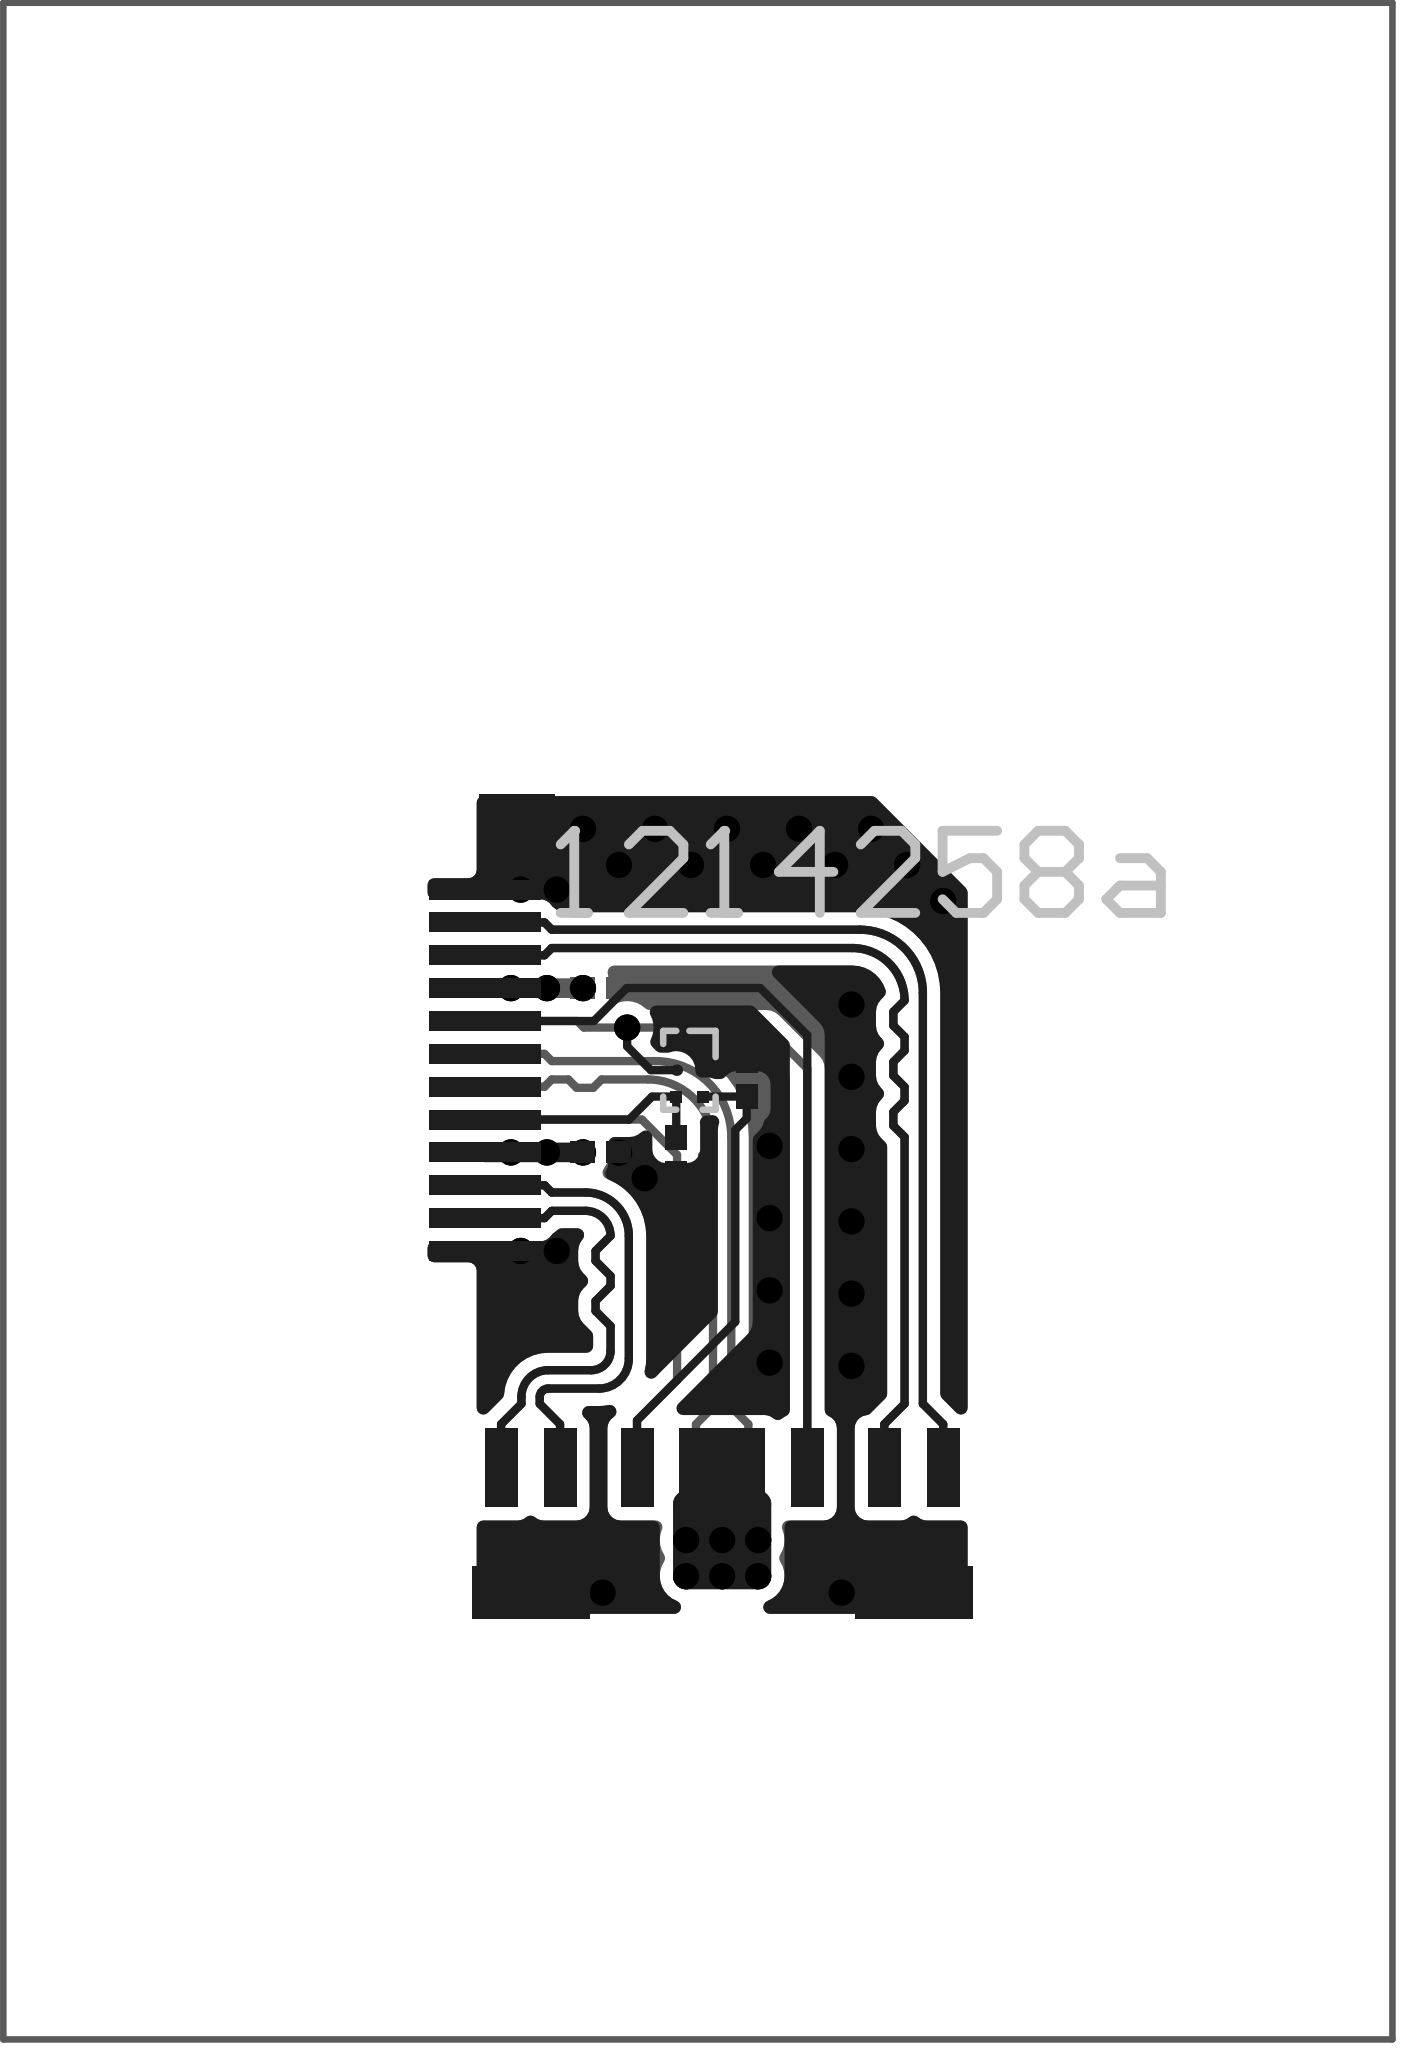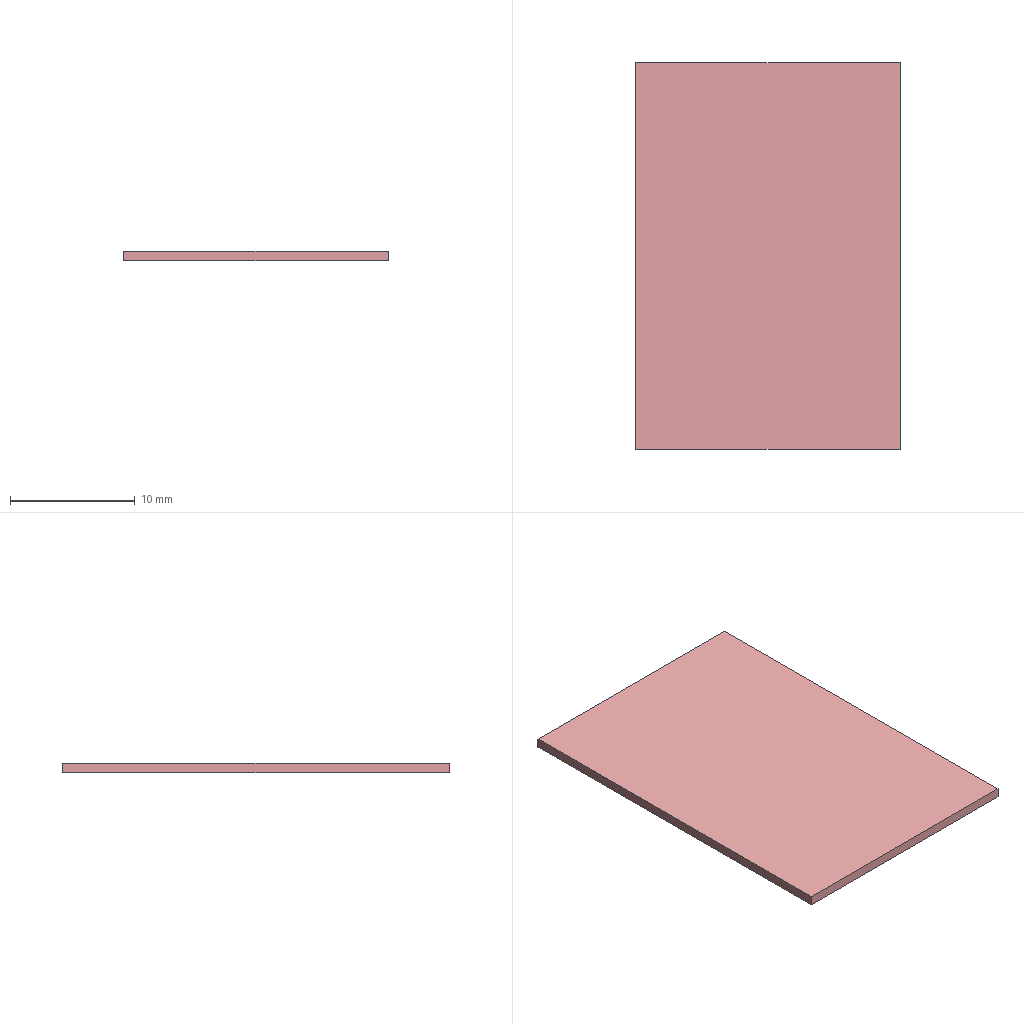Circuit board layout | Altium Designer | box 21.2 x 31 x 0.8 mm
Layer stack:
# Altium Designer layer stack of  (unit mm; dielectric type: 0 none, 1 core, 2 prepreg, 3 surface material)
index,name,kind,layer,copper_thickness_mm,dielectric_type,dielectric_thickness_mm,dielectric_material,dielectric_constant
0,Top Paste Mask Layer,other,,,,,,
1,Top Silkscreen Layer,other,,,,,,
2,Top Solder Mask Layer,dielectric,,,3,0.01,,0
3,Top Layer,copper,Top Layer,0.035,,,,
4,Dielectric1,dielectric,,,3,0.2133,7628 RC49% 8.6mil,0
5,Inner1,copper,Inner1,0.035,,,,
6,Dielectric2,dielectric,,,3,0.2133,1.1mm H/HOZ \u00BA\u00AC\u00CD\u00AD,0
7,Inner2,copper,Inner2,0.035,,,,
8,Dielectric3,dielectric,,,3,0.2133,7628 RC49% 8.6mil,0
9,Bottom Layer,copper,Bottom Layer,0.035,,,,
10,Bottom Solder Mask Layer,dielectric,,,3,0.01,,0
11,Bottom Silkscreen Layer,other,,,,,,
12,Bottom Paste Mask Layer,other,,,,,,
# drill layer pairs: low layer,high layer
drill_pair,Top Layer,Bottom Layer
Part placement:
Designator,Comment,Layer,Footprint,Center-X(mm),Center-Y(mm),Rotation
CN1,,TopLayer,简易版公头,77.45,84.6,90
U1,,TopLayer,wlcsp-6_l1.2-w0.8-r2-c3-p0.40-tl改,80.325,84.6,270
C1,,BottomLayer,c0201,78.974,85.85,0
C2,,TopLayer,c0201,78.974,83.35,0
C4,,TopLayer,c0201,81.2,84.474,90
C3,,TopLayer,c0201,80.124,83.301,270
Pad and via stacks:
# Altium Designer via and pad stacks of  (unit mm). Each distinct definition once, with the count of objects using it.
# via: kind,start_layer,end_layer,hole_mm,diameter_mm,mode(0 simple;1 top-mid-bottom;2 full stack),diameter_per_layer,count,example_net
# pad: kind,layer,hole_mm,hole_type(0 round;1 square;2 slot),plating,top_size,top_shape(1 round;2 rect;3 octagon;9 rounded rect),mid_size,bottom_size,mode,footprint,size_per_layer,count,example
pad,Bottom Layer,0,0,plated,0.5x1.2,2,0.5x1.2,0.5x1.2,0,,,8,7
pad,Bottom Layer,0,0,plated,0.8x1.8,2,0.8x1.8,0.8x1.8,0,,,2,7
pad,Bottom Layer,0,0,plated,1.05x1.15,2,1.05x1.15,1.05x1.15,0,\u00BC\u00F2\u00D2\u00D7\u00B0\u00E6\u00B9\u00AB\u00CD\u00B7,,2,CN1.A1
pad,Bottom Layer,0,0,plated,0.3x1.7,2,0.3x1.7,0.3x1.7,0,\u00BC\u00F2\u00D2\u00D7\u00B0\u00E6\u00B9\u00AB\u00CD\u00B7,,12,CN1.A2
pad,Bottom Layer,0,0,plated,0.3684x0.324,2,0.3684x0.324,0.3684x0.324,0,c0201,,2,C1.2
pad,Top Layer,0,0,plated,0.5x1.2,2,0.5x1.2,0.5x1.2,0,,,6,7
pad,Top Layer,0,0,plated,1.3x1.2,2,1.3x1.2,1.3x1.2,0,,,1,7
pad,Top Layer,0,0,plated,0.8x1.8,2,0.8x1.8,0.8x1.8,0,,,2,7
pad,Top Layer,0,0,plated,1.05x1.15,2,1.05x1.15,1.05x1.15,0,\u00BC\u00F2\u00D2\u00D7\u00B0\u00E6\u00B9\u00AB\u00CD\u00B7,,2,CN1.B1
pad,Top Layer,0,0,plated,0.3x1.7,2,0.3x1.7,0.3x1.7,0,\u00BC\u00F2\u00D2\u00D7\u00B0\u00E6\u00B9\u00AB\u00CD\u00B7,,12,CN1.B11
pad,Top Layer,0,0,plated,0.174x0.174,1,0.174x0.174,0.174x0.174,0,wlcsp-6_l1.2-w0.8-r2-c3-p0.40-tl\u00B8\u00C4,,4,U1.A1
pad,Top Layer,0,0,plated,0.174x0.174,2,0.174x0.174,0.174x0.174,0,wlcsp-6_l1.2-w0.8-r2-c3-p0.40-tl\u00B8\u00C4,,2,U1.C2
pad,Top Layer,0,0,plated,0.3684x0.324,2,0.3684x0.324,0.3684x0.324,0,c0201,,6,C2.2
via,Top Layer,Bottom Layer,0.2997,0.4,0,,50,GND
Copper pours:
name,layer,net,type(0 solid;1 hatched;2 none)
Bottom Layer-GND,Bottom Layer,GND,0
Inner1-GND,Inner1,GND,0
Top Layer-GND,Top Layer,GND,0
Inner2-VBUS,Inner2,VBUS,0
Design rules, without the lines most boards share:
# Altium Designer design rules of  (exported by Altium Designer, unit mm)
# columns: name | kind | enabled | priority | scope1 | scope2 | descriptor | typed fields (field=value)
otherClearance | 52 | enabled | 1 | All | All | Hole To Hole Clearance (Gap=11.8mil) (All),(All) | gap=0.2997
copperRegion | 20 | enabled | 1 | All | All | Polygon Connect Rule(Direct Connect )(Conductor Width=10mil) (Relief Angle=90 Angle) (Entries=4) (Air Gap Width=10mil) (All),(All) | connect_style(0=relief,1=direct,2=none)=1 relief_conductor_width=0.254 relief_entries=4
solderMaskExpansion | 13 | enabled | 2 | All | All | Solder Mask Expansion (Expansion =2.008mil) (All) | expansion=0.051